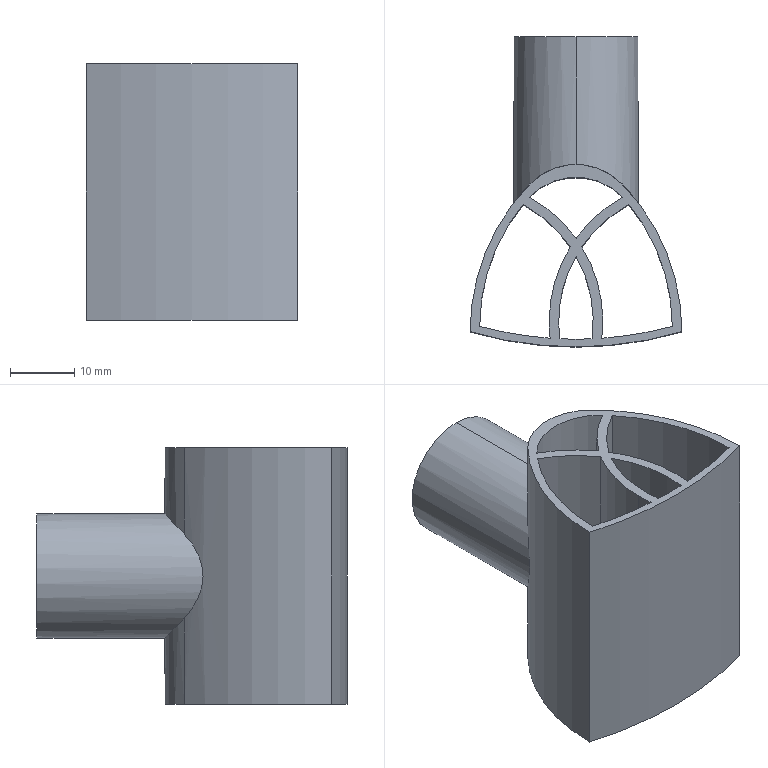Part | SolidWorks | features ICE 2, Extrusion 1 | 1 solid | 31 faces | box 33 x 48.321 x 40 mm | volume 10302 mm3 | cylinder 28 | plane 3 | commonest cylinder face diameters 41.207 x5 44.207 x5 20 x4 66 x4 114.5 x3 16 x2
STEP:
#1=CARTESIAN_POINT('',(-4.179,2.768,20.));
#2=VERTEX_POINT('',#1);
#3=CARTESIAN_POINT('',(-4.023,0.1415,20.));
#4=VERTEX_POINT('',#3);
#5=CARTESIAN_POINT('',(17.924,2.768,20.));
#6=DIRECTION('',(0.,0.,1.));
#7=DIRECTION('',(1.,0.,0.));
#8=AXIS2_PLACEMENT_3D('',#5,#6,#7);
#9=CIRCLE('',#8,22.103);
#10=EDGE_CURVE('',#2,#4,#9,.T.);
#11=ORIENTED_EDGE('',*,*,#10,.F.);
#12=CARTESIAN_POINT('',(-4.179,2.768,-20.));
#13=VERTEX_POINT('',#12);
#14=CARTESIAN_POINT('',(-4.179,2.768,20.));
#15=DIRECTION('',(0.,0.,-1.));
#16=VECTOR('',#15,1000.);
#17=LINE('',#14,#16);
#18=EDGE_CURVE('',#2,#13,#17,.T.);
#19=ORIENTED_EDGE('',*,*,#18,.T.);
#20=CARTESIAN_POINT('',(-4.023,0.1415,-20.));
#21=VERTEX_POINT('',#20);
#22=CARTESIAN_POINT('',(17.924,2.768,-20.));
#23=DIRECTION('',(0.,0.,1.));
#24=DIRECTION('',(1.,0.,0.));
#25=AXIS2_PLACEMENT_3D('',#22,#23,#24);
#26=CIRCLE('',#25,22.103);
#27=EDGE_CURVE('',#13,#21,#26,.T.);
#28=ORIENTED_EDGE('',*,*,#27,.T.);
#29=CARTESIAN_POINT('',(-4.023,0.1415,20.));
#30=DIRECTION('',(0.,0.,-1.));
#31=VECTOR('',#30,1000.);
#32=LINE('',#29,#31);
#33=EDGE_CURVE('',#4,#21,#32,.T.);
#34=ORIENTED_EDGE('',*,*,#33,.F.);
#35=EDGE_LOOP('',(#11,#19,#28,#34));
#36=FACE_OUTER_BOUND('',#35,.T.);
#37=CARTESIAN_POINT('',(17.924,2.768,20.));
#38=DIRECTION('',(0.,0.,-1.));
#39=DIRECTION('',(-1.,0.,0.));
#40=AXIS2_PLACEMENT_3D('',#37,#38,#39);
#41=CYLINDRICAL_SURFACE('',#40,22.103);
#42=ADVANCED_FACE('',(#36),#41,.T.);
#43=CARTESIAN_POINT('',(0.,12.928,20.));
#44=VERTEX_POINT('',#43);
#45=CARTESIAN_POINT('',(-2.679,2.768,20.));
#46=VERTEX_POINT('',#45);
#47=CARTESIAN_POINT('',(17.924,2.768,20.));
#48=DIRECTION('',(0.,0.,1.));
#49=DIRECTION('',(1.,0.,0.));
#50=AXIS2_PLACEMENT_3D('',#47,#48,#49);
#51=CIRCLE('',#50,20.603);
#52=EDGE_CURVE('',#44,#46,#51,.T.);
#53=ORIENTED_EDGE('',*,*,#52,.T.);
#54=CARTESIAN_POINT('',(-2.679,2.768,-20.));
#55=VERTEX_POINT('',#54);
#56=CARTESIAN_POINT('',(-2.679,2.768,20.));
#57=DIRECTION('',(0.,0.,-1.));
#58=VECTOR('',#57,1000.);
#59=LINE('',#56,#58);
#60=EDGE_CURVE('',#46,#55,#59,.T.);
#61=ORIENTED_EDGE('',*,*,#60,.T.);
#62=CARTESIAN_POINT('',(0.,12.928,-20.));
#63=VERTEX_POINT('',#62);
#64=CARTESIAN_POINT('',(17.924,2.768,-20.));
#65=DIRECTION('',(0.,0.,1.));
#66=DIRECTION('',(1.,0.,0.));
#67=AXIS2_PLACEMENT_3D('',#64,#65,#66);
#68=CIRCLE('',#67,20.603);
#69=EDGE_CURVE('',#63,#55,#68,.T.);
#70=ORIENTED_EDGE('',*,*,#69,.F.);
#71=CARTESIAN_POINT('',(0.,12.928,20.));
#72=DIRECTION('',(0.,0.,-1.));
#73=VECTOR('',#72,1000.);
#74=LINE('',#71,#73);
#75=EDGE_CURVE('',#44,#63,#74,.T.);
#76=ORIENTED_EDGE('',*,*,#75,.F.);
#77=EDGE_LOOP('',(#53,#61,#70,#76));
#78=FACE_OUTER_BOUND('',#77,.T.);
#79=CARTESIAN_POINT('',(17.924,2.768,20.));
#80=DIRECTION('',(0.,0.,-1.));
#81=DIRECTION('',(-1.,0.,0.));
#82=AXIS2_PLACEMENT_3D('',#79,#80,#81);
#83=CYLINDRICAL_SURFACE('',#82,20.603);
#84=ADVANCED_FACE('',(#78),#83,.F.);
#85=CARTESIAN_POINT('',(0.,27.201,-8.));
#86=VERTEX_POINT('',#85);
#87=CARTESIAN_POINT('',(-7.174,24.167,-3.54));
#88=VERTEX_POINT('',#87);
#89=CARTESIAN_POINT('',(0.,27.201,-8.));
#90=CARTESIAN_POINT('',(-0.3938,27.201,-8.));
#91=CARTESIAN_POINT('',(-0.7853,27.177,-7.971));
#92=CARTESIAN_POINT('',(-1.369,27.108,-7.884));
#93=CARTESIAN_POINT('',(-1.564,27.08,-7.848));
#94=CARTESIAN_POINT('',(-1.945,27.012,-7.762));
#95=CARTESIAN_POINT('',(-2.133,26.972,-7.713));
#96=CARTESIAN_POINT('',(-2.685,26.841,-7.546));
#97=CARTESIAN_POINT('',(-3.04,26.734,-7.41));
#98=CARTESIAN_POINT('',(-3.726,26.488,-7.089));
#99=CARTESIAN_POINT('',(-4.051,26.35,-6.908));
#100=CARTESIAN_POINT('',(-4.971,25.905,-6.311));
#101=CARTESIAN_POINT('',(-5.519,25.561,-5.835));
#102=CARTESIAN_POINT('',(-6.221,25.035,-5.042));
#103=CARTESIAN_POINT('',(-6.437,24.858,-4.764));
#104=CARTESIAN_POINT('',(-6.833,24.507,-4.176));
#105=CARTESIAN_POINT('',(-7.014,24.332,-3.865));
#106=CARTESIAN_POINT('',(-7.174,24.167,-3.54));
#107=B_SPLINE_CURVE_WITH_KNOTS('',3,(#89,#90,#91,#92,#93,#94,#95,#96,#97,#98,#99,#100,#101,#102,#103,#104,#105,#106),.UNSPECIFIED.,.F.,.F.,(4,2,2,2,2,2,2,2,4),(0.009445,0.01062,0.01121,0.0118,0.01297,0.01415,0.0165,0.01767,0.01885),.UNSPECIFIED.);
#108=EDGE_CURVE('',#86,#88,#107,.T.);
#109=ORIENTED_EDGE('',*,*,#108,.F.);
#110=CARTESIAN_POINT('',(0.,47.121,-8.));
#111=VERTEX_POINT('',#110);
#112=CARTESIAN_POINT('',(0.,-1.201,-8.));
#113=DIRECTION('',(0.,1.,0.));
#114=VECTOR('',#113,1000.);
#115=LINE('',#112,#114);
#116=EDGE_CURVE('',#86,#111,#115,.T.);
#117=ORIENTED_EDGE('',*,*,#116,.T.);
#118=CARTESIAN_POINT('',(0.,47.121,8.));
#119=VERTEX_POINT('',#118);
#120=CARTESIAN_POINT('',(0.,47.121,0.));
#121=DIRECTION('',(0.,-1.,0.));
#122=DIRECTION('',(0.,0.,-1.));
#123=AXIS2_PLACEMENT_3D('',#120,#121,#122);
#124=CIRCLE('',#123,8.);
#125=EDGE_CURVE('',#119,#111,#124,.T.);
#126=ORIENTED_EDGE('',*,*,#125,.F.);
#127=CARTESIAN_POINT('',(0.,27.201,8.));
#128=VERTEX_POINT('',#127);
#129=CARTESIAN_POINT('',(0.,-1.201,8.));
#130=DIRECTION('',(0.,1.,0.));
#131=VECTOR('',#130,1000.);
#132=LINE('',#129,#131);
#133=EDGE_CURVE('',#128,#119,#132,.T.);
#134=ORIENTED_EDGE('',*,*,#133,.F.);
#135=CARTESIAN_POINT('',(-7.174,24.167,3.54));
#136=VERTEX_POINT('',#135);
#137=CARTESIAN_POINT('',(-7.174,24.167,3.54));
#138=CARTESIAN_POINT('',(-6.852,24.498,4.192));
#139=CARTESIAN_POINT('',(-6.459,24.857,4.773));
#140=CARTESIAN_POINT('',(-5.756,25.383,5.567));
#141=CARTESIAN_POINT('',(-5.501,25.558,5.82));
#142=CARTESIAN_POINT('',(-4.956,25.892,6.29));
#143=CARTESIAN_POINT('',(-4.668,26.051,6.507));
#144=CARTESIAN_POINT('',(-4.059,26.346,6.903));
#145=CARTESIAN_POINT('',(-3.738,26.483,7.083));
#146=CARTESIAN_POINT('',(-3.059,26.728,7.402));
#147=CARTESIAN_POINT('',(-2.697,26.838,7.542));
#148=CARTESIAN_POINT('',(-1.957,27.015,7.767));
#149=CARTESIAN_POINT('',(-1.577,27.083,7.853));
#150=CARTESIAN_POINT('',(-0.7976,27.177,7.97));
#151=CARTESIAN_POINT('',(-0.3955,27.201,8.));
#152=CARTESIAN_POINT('',(0.,27.201,8.));
#153=B_SPLINE_CURVE_WITH_KNOTS('',3,(#137,#138,#139,#140,#141,#142,#143,#144,#145,#146,#147,#148,#149,#150,#151,#152),.UNSPECIFIED.,.F.,.F.,(4,2,2,2,2,2,2,4),(0.,0.002361,0.003542,0.004722,0.005903,0.007083,0.008264,0.009445),.UNSPECIFIED.);
#154=EDGE_CURVE('',#136,#128,#153,.T.);
#155=ORIENTED_EDGE('',*,*,#154,.F.);
#156=CARTESIAN_POINT('',(-7.174,24.167,3.54));
#157=CARTESIAN_POINT('',(-7.431,23.903,3.02));
#158=CARTESIAN_POINT('',(-7.636,23.683,2.465));
#159=CARTESIAN_POINT('',(-7.852,23.449,1.565));
#160=CARTESIAN_POINT('',(-7.907,23.388,1.256));
#161=CARTESIAN_POINT('',(-7.981,23.306,0.6372));
#162=CARTESIAN_POINT('',(-8.,23.285,0.324));
#163=CARTESIAN_POINT('',(-8.,23.285,-0.3096));
#164=CARTESIAN_POINT('',(-7.981,23.306,-0.6302));
#165=CARTESIAN_POINT('',(-7.908,23.387,-1.252));
#166=CARTESIAN_POINT('',(-7.853,23.447,-1.557));
#167=CARTESIAN_POINT('',(-7.71,23.602,-2.156));
#168=CARTESIAN_POINT('',(-7.622,23.698,-2.449));
#169=CARTESIAN_POINT('',(-7.418,23.914,-3.01));
#170=CARTESIAN_POINT('',(-7.302,24.035,-3.28));
#171=CARTESIAN_POINT('',(-7.174,24.167,-3.54));
#172=B_SPLINE_CURVE_WITH_KNOTS('',3,(#156,#157,#158,#159,#160,#161,#162,#163,#164,#165,#166,#167,#168,#169,#170,#171),.UNSPECIFIED.,.F.,.F.,(4,2,2,2,2,2,2,4),(0.,0.001893,0.00284,0.003787,0.004734,0.00568,0.006627,0.007574),.UNSPECIFIED.);
#173=EDGE_CURVE('',#136,#88,#172,.T.);
#174=ORIENTED_EDGE('',*,*,#173,.T.);
#175=EDGE_LOOP('',(#109,#117,#126,#134,#155,#174));
#176=FACE_OUTER_BOUND('',#175,.T.);
#177=CARTESIAN_POINT('',(0.,-1.201,0.));
#178=DIRECTION('',(0.,1.,0.));
#179=DIRECTION('',(0.,0.,1.));
#180=AXIS2_PLACEMENT_3D('',#177,#178,#179);
#181=CYLINDRICAL_SURFACE('',#180,8.);
#182=ADVANCED_FACE('',(#176),#181,.F.);
#183=CARTESIAN_POINT('',(7.174,24.167,-6.529));
#184=VERTEX_POINT('',#183);
#185=CARTESIAN_POINT('',(0.,27.201,-9.7));
#186=VERTEX_POINT('',#185);
#187=CARTESIAN_POINT('',(7.174,24.167,-6.529));
#188=CARTESIAN_POINT('',(6.767,24.586,-6.976));
#189=CARTESIAN_POINT('',(6.315,24.98,-7.39));
#190=CARTESIAN_POINT('',(5.556,25.521,-7.958));
#191=CARTESIAN_POINT('',(5.289,25.694,-8.138));
#192=CARTESIAN_POINT('',(4.725,26.02,-8.478));
#193=CARTESIAN_POINT('',(4.429,26.173,-8.636));
#194=CARTESIAN_POINT('',(3.818,26.449,-8.923));
#195=CARTESIAN_POINT('',(3.501,26.574,-9.053));
#196=CARTESIAN_POINT('',(2.844,26.794,-9.28));
#197=CARTESIAN_POINT('',(2.5,26.89,-9.379));
#198=CARTESIAN_POINT('',(1.45,27.121,-9.618));
#199=CARTESIAN_POINT('',(0.7337,27.201,-9.7));
#200=CARTESIAN_POINT('',(0.,27.201,-9.7));
#201=B_SPLINE_CURVE_WITH_KNOTS('',3,(#187,#188,#189,#190,#191,#192,#193,#194,#195,#196,#197,#198,#199,#200),.UNSPECIFIED.,.F.,.F.,(4,2,2,2,2,2,4),(0.,0.002182,0.003273,0.004364,0.005455,0.006546,0.008728),.UNSPECIFIED.);
#202=EDGE_CURVE('',#184,#186,#201,.T.);
#203=ORIENTED_EDGE('',*,*,#202,.T.);
#204=CARTESIAN_POINT('',(0.,47.121,-9.7));
#205=VERTEX_POINT('',#204);
#206=CARTESIAN_POINT('',(0.,-1.201,-9.7));
#207=DIRECTION('',(0.,1.,0.));
#208=VECTOR('',#207,1000.);
#209=LINE('',#206,#208);
#210=EDGE_CURVE('',#186,#205,#209,.T.);
#211=ORIENTED_EDGE('',*,*,#210,.T.);
#212=CARTESIAN_POINT('',(0.,47.121,9.7));
#213=VERTEX_POINT('',#212);
#214=CARTESIAN_POINT('',(0.,47.121,0.));
#215=DIRECTION('',(0.,-1.,0.));
#216=DIRECTION('',(0.,0.,-1.));
#217=AXIS2_PLACEMENT_3D('',#214,#215,#216);
#218=CIRCLE('',#217,9.7);
#219=EDGE_CURVE('',#205,#213,#218,.T.);
#220=ORIENTED_EDGE('',*,*,#219,.T.);
#221=CARTESIAN_POINT('',(0.,27.201,9.7));
#222=VERTEX_POINT('',#221);
#223=CARTESIAN_POINT('',(0.,-1.201,9.7));
#224=DIRECTION('',(0.,1.,0.));
#225=VECTOR('',#224,1000.);
#226=LINE('',#223,#225);
#227=EDGE_CURVE('',#222,#213,#226,.T.);
#228=ORIENTED_EDGE('',*,*,#227,.F.);
#229=CARTESIAN_POINT('',(7.174,24.167,6.529));
#230=VERTEX_POINT('',#229);
#231=CARTESIAN_POINT('',(0.,27.201,9.7));
#232=CARTESIAN_POINT('',(0.366,27.201,9.7));
#233=CARTESIAN_POINT('',(0.7354,27.18,9.679));
#234=CARTESIAN_POINT('',(1.455,27.101,9.597));
#235=CARTESIAN_POINT('',(1.809,27.042,9.537));
#236=CARTESIAN_POINT('',(2.505,26.888,9.378));
#237=CARTESIAN_POINT('',(2.849,26.792,9.279));
#238=CARTESIAN_POINT('',(3.508,26.572,9.05));
#239=CARTESIAN_POINT('',(3.825,26.446,8.92));
#240=CARTESIAN_POINT('',(4.436,26.169,8.633));
#241=CARTESIAN_POINT('',(4.732,26.016,8.474));
#242=CARTESIAN_POINT('',(5.294,25.691,8.135));
#243=CARTESIAN_POINT('',(5.559,25.519,7.955));
#244=CARTESIAN_POINT('',(6.316,24.978,7.389));
#245=CARTESIAN_POINT('',(6.768,24.586,6.975));
#246=CARTESIAN_POINT('',(7.174,24.167,6.529));
#247=B_SPLINE_CURVE_WITH_KNOTS('',3,(#231,#232,#233,#234,#235,#236,#237,#238,#239,#240,#241,#242,#243,#244,#245,#246),.UNSPECIFIED.,.F.,.F.,(4,2,2,2,2,2,2,4),(0.008728,0.009816,0.0109,0.01199,0.01308,0.01417,0.01526,0.01743),.UNSPECIFIED.);
#248=EDGE_CURVE('',#222,#230,#247,.T.);
#249=ORIENTED_EDGE('',*,*,#248,.T.);
#250=CARTESIAN_POINT('',(7.174,24.167,6.529));
#251=CARTESIAN_POINT('',(7.538,23.793,6.129));
#252=CARTESIAN_POINT('',(7.87,23.433,5.697));
#253=CARTESIAN_POINT('',(8.32,22.926,4.994));
#254=CARTESIAN_POINT('',(8.462,22.763,4.75));
#255=CARTESIAN_POINT('',(8.729,22.45,4.24));
#256=CARTESIAN_POINT('',(8.854,22.301,3.973));
#257=CARTESIAN_POINT('',(9.195,21.888,3.147));
#258=CARTESIAN_POINT('',(9.377,21.657,2.564));
#259=CARTESIAN_POINT('',(9.568,21.412,1.624));
#260=CARTESIAN_POINT('',(9.617,21.349,1.304));
#261=CARTESIAN_POINT('',(9.683,21.264,0.6603));
#262=CARTESIAN_POINT('',(9.7,21.241,0.3346));
#263=CARTESIAN_POINT('',(9.7,21.241,-0.3247));
#264=CARTESIAN_POINT('',(9.683,21.263,-0.6547));
#265=CARTESIAN_POINT('',(9.618,21.348,-1.299));
#266=CARTESIAN_POINT('',(9.57,21.41,-1.617));
#267=CARTESIAN_POINT('',(9.443,21.573,-2.241));
#268=CARTESIAN_POINT('',(9.364,21.672,-2.548));
#269=CARTESIAN_POINT('',(9.185,21.897,-3.134));
#270=CARTESIAN_POINT('',(9.083,22.023,-3.417));
#271=CARTESIAN_POINT('',(8.745,22.433,-4.239));
#272=CARTESIAN_POINT('',(8.474,22.753,-4.753));
#273=CARTESIAN_POINT('',(7.871,23.431,-5.696));
#274=CARTESIAN_POINT('',(7.538,23.792,-6.129));
#275=CARTESIAN_POINT('',(7.174,24.167,-6.529));
#276=B_SPLINE_CURVE_WITH_KNOTS('',3,(#250,#251,#252,#253,#254,#255,#256,#257,#258,#259,#260,#261,#262,#263,#264,#265,#266,#267,#268,#269,#270,#271,#272,#273,#274,#275),.UNSPECIFIED.,.F.,.F.,(4,2,2,2,2,2,2,2,2,2,2,2,4),(0.,0.001953,0.00293,0.003907,0.00586,0.006837,0.007814,0.008791,0.009767,0.01074,0.01172,0.01367,0.01563),.UNSPECIFIED.);
#277=EDGE_CURVE('',#230,#184,#276,.T.);
#278=ORIENTED_EDGE('',*,*,#277,.T.);
#279=EDGE_LOOP('',(#203,#211,#220,#228,#249,#278));
#280=FACE_OUTER_BOUND('',#279,.T.);
#281=CARTESIAN_POINT('',(0.,-1.201,0.));
#282=DIRECTION('',(0.,1.,0.));
#283=DIRECTION('',(0.,0.,1.));
#284=AXIS2_PLACEMENT_3D('',#281,#282,#283);
#285=CYLINDRICAL_SURFACE('',#284,9.7);
#286=ADVANCED_FACE('',(#280),#285,.T.);
#287=ORIENTED_EDGE('',*,*,#277,.F.);
#288=CARTESIAN_POINT('',(7.174,24.167,20.));
#289=VERTEX_POINT('',#288);
#290=CARTESIAN_POINT('',(7.174,24.167,20.));
#291=DIRECTION('',(0.,0.,-1.));
#292=VECTOR('',#291,1000.);
#293=LINE('',#290,#292);
#294=EDGE_CURVE('',#289,#230,#293,.T.);
#295=ORIENTED_EDGE('',*,*,#294,.F.);
#296=CARTESIAN_POINT('',(16.5,1.177,20.));
#297=VERTEX_POINT('',#296);
#298=CARTESIAN_POINT('',(-16.5,1.177,20.));
#299=DIRECTION('',(0.,0.,1.));
#300=DIRECTION('',(1.,0.,0.));
#301=AXIS2_PLACEMENT_3D('',#298,#299,#300);
#302=CIRCLE('',#301,33.);
#303=EDGE_CURVE('',#297,#289,#302,.T.);
#304=ORIENTED_EDGE('',*,*,#303,.F.);
#305=CARTESIAN_POINT('',(16.5,1.177,-20.));
#306=VERTEX_POINT('',#305);
#307=CARTESIAN_POINT('',(16.5,1.177,20.));
#308=DIRECTION('',(0.,0.,-1.));
#309=VECTOR('',#308,1000.);
#310=LINE('',#307,#309);
#311=EDGE_CURVE('',#297,#306,#310,.T.);
#312=ORIENTED_EDGE('',*,*,#311,.T.);
#313=CARTESIAN_POINT('',(7.174,24.167,-20.));
#314=VERTEX_POINT('',#313);
#315=CARTESIAN_POINT('',(-16.5,1.177,-20.));
#316=DIRECTION('',(0.,0.,1.));
#317=DIRECTION('',(1.,0.,0.));
#318=AXIS2_PLACEMENT_3D('',#315,#316,#317);
#319=CIRCLE('',#318,33.);
#320=EDGE_CURVE('',#306,#314,#319,.T.);
#321=ORIENTED_EDGE('',*,*,#320,.T.);
#322=CARTESIAN_POINT('',(7.174,24.167,20.));
#323=DIRECTION('',(0.,0.,-1.));
#324=VECTOR('',#323,1000.);
#325=LINE('',#322,#324);
#326=EDGE_CURVE('',#184,#314,#325,.T.);
#327=ORIENTED_EDGE('',*,*,#326,.F.);
#328=EDGE_LOOP('',(#287,#295,#304,#312,#321,#327));
#329=FACE_OUTER_BOUND('',#328,.T.);
#330=CARTESIAN_POINT('',(-16.5,1.177,20.));
#331=DIRECTION('',(0.,0.,-1.));
#332=DIRECTION('',(-1.,0.,0.));
#333=AXIS2_PLACEMENT_3D('',#330,#331,#332);
#334=CYLINDRICAL_SURFACE('',#333,33.);
#335=ADVANCED_FACE('',(#329),#334,.T.);
#336=ORIENTED_EDGE('',*,*,#202,.F.);
#337=ORIENTED_EDGE('',*,*,#326,.T.);
#338=CARTESIAN_POINT('',(-7.174,24.167,-20.));
#339=VERTEX_POINT('',#338);
#340=CARTESIAN_POINT('',(0.,17.201,-20.));
#341=DIRECTION('',(0.,0.,1.));
#342=DIRECTION('',(1.,0.,0.));
#343=AXIS2_PLACEMENT_3D('',#340,#341,#342);
#344=CIRCLE('',#343,10.);
#345=EDGE_CURVE('',#314,#339,#344,.T.);
#346=ORIENTED_EDGE('',*,*,#345,.T.);
#347=CARTESIAN_POINT('',(-7.174,24.167,-6.529));
#348=VERTEX_POINT('',#347);
#349=CARTESIAN_POINT('',(-7.174,24.167,20.));
#350=DIRECTION('',(0.,0.,-1.));
#351=VECTOR('',#350,1000.);
#352=LINE('',#349,#351);
#353=EDGE_CURVE('',#348,#339,#352,.T.);
#354=ORIENTED_EDGE('',*,*,#353,.F.);
#355=CARTESIAN_POINT('',(0.,27.201,-9.7));
#356=CARTESIAN_POINT('',(-0.366,27.201,-9.7));
#357=CARTESIAN_POINT('',(-0.7354,27.18,-9.679));
#358=CARTESIAN_POINT('',(-1.455,27.101,-9.597));
#359=CARTESIAN_POINT('',(-1.809,27.042,-9.537));
#360=CARTESIAN_POINT('',(-2.505,26.888,-9.378));
#361=CARTESIAN_POINT('',(-2.849,26.792,-9.279));
#362=CARTESIAN_POINT('',(-3.508,26.572,-9.05));
#363=CARTESIAN_POINT('',(-3.825,26.446,-8.92));
#364=CARTESIAN_POINT('',(-4.436,26.169,-8.633));
#365=CARTESIAN_POINT('',(-4.732,26.016,-8.474));
#366=CARTESIAN_POINT('',(-5.294,25.691,-8.135));
#367=CARTESIAN_POINT('',(-5.559,25.519,-7.955));
#368=CARTESIAN_POINT('',(-6.316,24.978,-7.389));
#369=CARTESIAN_POINT('',(-6.768,24.586,-6.975));
#370=CARTESIAN_POINT('',(-7.174,24.167,-6.529));
#371=B_SPLINE_CURVE_WITH_KNOTS('',3,(#355,#356,#357,#358,#359,#360,#361,#362,#363,#364,#365,#366,#367,#368,#369,#370),.UNSPECIFIED.,.F.,.F.,(4,2,2,2,2,2,2,4),(0.008728,0.009816,0.0109,0.01199,0.01308,0.01417,0.01526,0.01743),.UNSPECIFIED.);
#372=EDGE_CURVE('',#186,#348,#371,.T.);
#373=ORIENTED_EDGE('',*,*,#372,.F.);
#374=EDGE_LOOP('',(#336,#337,#346,#354,#373));
#375=FACE_OUTER_BOUND('',#374,.T.);
#376=CARTESIAN_POINT('',(0.,17.201,20.));
#377=DIRECTION('',(0.,0.,-1.));
#378=DIRECTION('',(-1.,0.,0.));
#379=AXIS2_PLACEMENT_3D('',#376,#377,#378);
#380=CYLINDRICAL_SURFACE('',#379,10.);
#381=ADVANCED_FACE('',(#375),#380,.T.);
#382=CARTESIAN_POINT('',(-7.174,24.167,6.529));
#383=VERTEX_POINT('',#382);
#384=CARTESIAN_POINT('',(-7.174,24.167,6.529));
#385=CARTESIAN_POINT('',(-6.767,24.586,6.976));
#386=CARTESIAN_POINT('',(-6.315,24.98,7.39));
#387=CARTESIAN_POINT('',(-5.556,25.521,7.958));
#388=CARTESIAN_POINT('',(-5.289,25.694,8.138));
#389=CARTESIAN_POINT('',(-4.725,26.02,8.478));
#390=CARTESIAN_POINT('',(-4.429,26.173,8.636));
#391=CARTESIAN_POINT('',(-3.818,26.449,8.923));
#392=CARTESIAN_POINT('',(-3.501,26.574,9.053));
#393=CARTESIAN_POINT('',(-2.844,26.794,9.28));
#394=CARTESIAN_POINT('',(-2.5,26.89,9.379));
#395=CARTESIAN_POINT('',(-1.45,27.121,9.618));
#396=CARTESIAN_POINT('',(-0.7337,27.201,9.7));
#397=CARTESIAN_POINT('',(0.,27.201,9.7));
#398=B_SPLINE_CURVE_WITH_KNOTS('',3,(#384,#385,#386,#387,#388,#389,#390,#391,#392,#393,#394,#395,#396,#397),.UNSPECIFIED.,.F.,.F.,(4,2,2,2,2,2,4),(0.,0.002182,0.003273,0.004364,0.005455,0.006546,0.008728),.UNSPECIFIED.);
#399=EDGE_CURVE('',#383,#222,#398,.T.);
#400=ORIENTED_EDGE('',*,*,#399,.F.);
#401=CARTESIAN_POINT('',(-7.174,24.167,20.));
#402=VERTEX_POINT('',#401);
#403=CARTESIAN_POINT('',(-7.174,24.167,20.));
#404=DIRECTION('',(0.,0.,-1.));
#405=VECTOR('',#404,1000.);
#406=LINE('',#403,#405);
#407=EDGE_CURVE('',#402,#383,#406,.T.);
#408=ORIENTED_EDGE('',*,*,#407,.F.);
#409=CARTESIAN_POINT('',(0.,17.201,20.));
#410=DIRECTION('',(0.,0.,1.));
#411=DIRECTION('',(1.,0.,0.));
#412=AXIS2_PLACEMENT_3D('',#409,#410,#411);
#413=CIRCLE('',#412,10.);
#414=EDGE_CURVE('',#289,#402,#413,.T.);
#415=ORIENTED_EDGE('',*,*,#414,.F.);
#416=ORIENTED_EDGE('',*,*,#294,.T.);
#417=ORIENTED_EDGE('',*,*,#248,.F.);
#418=EDGE_LOOP('',(#400,#408,#415,#416,#417));
#419=FACE_OUTER_BOUND('',#418,.T.);
#420=CARTESIAN_POINT('',(0.,17.201,20.));
#421=DIRECTION('',(0.,0.,-1.));
#422=DIRECTION('',(-1.,0.,0.));
#423=AXIS2_PLACEMENT_3D('',#420,#421,#422);
#424=CYLINDRICAL_SURFACE('',#423,10.);
#425=ADVANCED_FACE('',(#419),#424,.T.);
#426=ORIENTED_EDGE('',*,*,#407,.T.);
#427=CARTESIAN_POINT('',(-7.174,24.167,6.529));
#428=CARTESIAN_POINT('',(-7.538,23.793,6.129));
#429=CARTESIAN_POINT('',(-7.87,23.433,5.697));
#430=CARTESIAN_POINT('',(-8.32,22.926,4.994));
#431=CARTESIAN_POINT('',(-8.462,22.763,4.75));
#432=CARTESIAN_POINT('',(-8.729,22.45,4.24));
#433=CARTESIAN_POINT('',(-8.854,22.301,3.973));
#434=CARTESIAN_POINT('',(-9.195,21.888,3.147));
#435=CARTESIAN_POINT('',(-9.377,21.657,2.564));
#436=CARTESIAN_POINT('',(-9.568,21.412,1.624));
#437=CARTESIAN_POINT('',(-9.617,21.349,1.304));
#438=CARTESIAN_POINT('',(-9.683,21.264,0.6603));
#439=CARTESIAN_POINT('',(-9.7,21.241,0.3346));
#440=CARTESIAN_POINT('',(-9.7,21.241,-0.3247));
#441=CARTESIAN_POINT('',(-9.683,21.263,-0.6547));
#442=CARTESIAN_POINT('',(-9.618,21.348,-1.299));
#443=CARTESIAN_POINT('',(-9.57,21.41,-1.617));
#444=CARTESIAN_POINT('',(-9.443,21.573,-2.241));
#445=CARTESIAN_POINT('',(-9.364,21.672,-2.548));
#446=CARTESIAN_POINT('',(-9.185,21.897,-3.134));
#447=CARTESIAN_POINT('',(-9.083,22.023,-3.417));
#448=CARTESIAN_POINT('',(-8.745,22.433,-4.239));
#449=CARTESIAN_POINT('',(-8.474,22.753,-4.753));
#450=CARTESIAN_POINT('',(-7.871,23.431,-5.696));
#451=CARTESIAN_POINT('',(-7.538,23.792,-6.129));
#452=CARTESIAN_POINT('',(-7.174,24.167,-6.529));
#453=B_SPLINE_CURVE_WITH_KNOTS('',3,(#427,#428,#429,#430,#431,#432,#433,#434,#435,#436,#437,#438,#439,#440,#441,#442,#443,#444,#445,#446,#447,#448,#449,#450,#451,#452),.UNSPECIFIED.,.F.,.F.,(4,2,2,2,2,2,2,2,2,2,2,2,4),(0.,0.001953,0.00293,0.003907,0.00586,0.006837,0.007814,0.008791,0.009767,0.01074,0.01172,0.01367,0.01563),.UNSPECIFIED.);
#454=EDGE_CURVE('',#383,#348,#453,.T.);
#455=ORIENTED_EDGE('',*,*,#454,.T.);
#456=ORIENTED_EDGE('',*,*,#353,.T.);
#457=CARTESIAN_POINT('',(-16.5,1.177,-20.));
#458=VERTEX_POINT('',#457);
#459=CARTESIAN_POINT('',(16.5,1.177,-20.));
#460=DIRECTION('',(0.,0.,-1.));
#461=DIRECTION('',(1.,0.,0.));
#462=AXIS2_PLACEMENT_3D('',#459,#460,#461);
#463=CIRCLE('',#462,33.);
#464=EDGE_CURVE('',#458,#339,#463,.T.);
#465=ORIENTED_EDGE('',*,*,#464,.F.);
#466=CARTESIAN_POINT('',(-16.5,1.177,20.));
#467=VERTEX_POINT('',#466);
#468=CARTESIAN_POINT('',(-16.5,1.177,20.));
#469=DIRECTION('',(0.,0.,-1.));
#470=VECTOR('',#469,1000.);
#471=LINE('',#468,#470);
#472=EDGE_CURVE('',#467,#458,#471,.T.);
#473=ORIENTED_EDGE('',*,*,#472,.F.);
#474=CARTESIAN_POINT('',(16.5,1.177,20.));
#475=DIRECTION('',(0.,0.,-1.));
#476=DIRECTION('',(1.,0.,0.));
#477=AXIS2_PLACEMENT_3D('',#474,#475,#476);
#478=CIRCLE('',#477,33.);
#479=EDGE_CURVE('',#467,#402,#478,.T.);
#480=ORIENTED_EDGE('',*,*,#479,.T.);
#481=EDGE_LOOP('',(#426,#455,#456,#465,#473,#480));
#482=FACE_OUTER_BOUND('',#481,.T.);
#483=CARTESIAN_POINT('',(16.5,1.177,20.));
#484=DIRECTION('',(0.,0.,-1.));
#485=DIRECTION('',(-1.,0.,0.));
#486=AXIS2_PLACEMENT_3D('',#483,#484,#485);
#487=CYLINDRICAL_SURFACE('',#486,33.);
#488=ADVANCED_FACE('',(#482),#487,.T.);
#489=CARTESIAN_POINT('',(-15.,2.,-20.));
#490=VERTEX_POINT('',#489);
#491=CARTESIAN_POINT('',(-8.25,20.959,-20.));
#492=VERTEX_POINT('',#491);
#493=CARTESIAN_POINT('',(15.,2.,-20.));
#494=DIRECTION('',(0.,0.,-1.));
#495=DIRECTION('',(1.,0.,0.));
#496=AXIS2_PLACEMENT_3D('',#493,#494,#495);
#497=CIRCLE('',#496,30.);
#498=EDGE_CURVE('',#490,#492,#497,.T.);
#499=ORIENTED_EDGE('',*,*,#498,.T.);
#500=CARTESIAN_POINT('',(-8.25,20.959,20.));
#501=VERTEX_POINT('',#500);
#502=CARTESIAN_POINT('',(-8.25,20.959,20.));
#503=DIRECTION('',(0.,0.,-1.));
#504=VECTOR('',#503,1000.);
#505=LINE('',#502,#504);
#506=EDGE_CURVE('',#501,#492,#505,.T.);
#507=ORIENTED_EDGE('',*,*,#506,.F.);
#508=CARTESIAN_POINT('',(-15.,2.,20.));
#509=VERTEX_POINT('',#508);
#510=CARTESIAN_POINT('',(15.,2.,20.));
#511=DIRECTION('',(0.,0.,-1.));
#512=DIRECTION('',(1.,0.,0.));
#513=AXIS2_PLACEMENT_3D('',#510,#511,#512);
#514=CIRCLE('',#513,30.);
#515=EDGE_CURVE('',#509,#501,#514,.T.);
#516=ORIENTED_EDGE('',*,*,#515,.F.);
#517=CARTESIAN_POINT('',(-15.,2.,20.));
#518=DIRECTION('',(0.,0.,-1.));
#519=VECTOR('',#518,1000.);
#520=LINE('',#517,#519);
#521=EDGE_CURVE('',#509,#490,#520,.T.);
#522=ORIENTED_EDGE('',*,*,#521,.T.);
#523=EDGE_LOOP('',(#499,#507,#516,#522));
#524=FACE_OUTER_BOUND('',#523,.T.);
#525=CARTESIAN_POINT('',(15.,2.,20.));
#526=DIRECTION('',(0.,0.,-1.));
#527=DIRECTION('',(-1.,0.,0.));
#528=AXIS2_PLACEMENT_3D('',#525,#526,#527);
#529=CYLINDRICAL_SURFACE('',#528,30.);
#530=ADVANCED_FACE('',(#524),#529,.F.);
#531=CARTESIAN_POINT('',(8.25,20.959,20.));
#532=VERTEX_POINT('',#531);
#533=CARTESIAN_POINT('',(8.25,20.959,-20.));
#534=VERTEX_POINT('',#533);
#535=CARTESIAN_POINT('',(8.25,20.959,20.));
#536=DIRECTION('',(0.,0.,-1.));
#537=VECTOR('',#536,1000.);
#538=LINE('',#535,#537);
#539=EDGE_CURVE('',#532,#534,#538,.T.);
#540=ORIENTED_EDGE('',*,*,#539,.T.);
#541=CARTESIAN_POINT('',(15.,2.,-20.));
#542=VERTEX_POINT('',#541);
#543=CARTESIAN_POINT('',(-15.,2.,-20.));
#544=DIRECTION('',(0.,0.,1.));
#545=DIRECTION('',(1.,0.,0.));
#546=AXIS2_PLACEMENT_3D('',#543,#544,#545);
#547=CIRCLE('',#546,30.);
#548=EDGE_CURVE('',#542,#534,#547,.T.);
#549=ORIENTED_EDGE('',*,*,#548,.F.);
#550=CARTESIAN_POINT('',(15.,2.,20.));
#551=VERTEX_POINT('',#550);
#552=CARTESIAN_POINT('',(15.,2.,20.));
#553=DIRECTION('',(0.,0.,-1.));
#554=VECTOR('',#553,1000.);
#555=LINE('',#552,#554);
#556=EDGE_CURVE('',#551,#542,#555,.T.);
#557=ORIENTED_EDGE('',*,*,#556,.F.);
#558=CARTESIAN_POINT('',(-15.,2.,20.));
#559=DIRECTION('',(0.,0.,1.));
#560=DIRECTION('',(1.,0.,0.));
#561=AXIS2_PLACEMENT_3D('',#558,#559,#560);
#562=CIRCLE('',#561,30.);
#563=EDGE_CURVE('',#551,#532,#562,.T.);
#564=ORIENTED_EDGE('',*,*,#563,.T.);
#565=EDGE_LOOP('',(#540,#549,#557,#564));
#566=FACE_OUTER_BOUND('',#565,.T.);
#567=CARTESIAN_POINT('',(-15.,2.,20.));
#568=DIRECTION('',(0.,0.,-1.));
#569=DIRECTION('',(-1.,0.,0.));
#570=AXIS2_PLACEMENT_3D('',#567,#568,#569);
#571=CYLINDRICAL_SURFACE('',#570,30.);
#572=ADVANCED_FACE('',(#566),#571,.F.);
#573=CARTESIAN_POINT('',(0.,57.25,-20.));
#574=DIRECTION('',(0.,0.,1.));
#575=DIRECTION('',(1.,0.,0.));
#576=AXIS2_PLACEMENT_3D('',#573,#574,#575);
#577=CIRCLE('',#576,58.45);
#578=EDGE_CURVE('',#458,#306,#577,.T.);
#579=ORIENTED_EDGE('',*,*,#578,.T.);
#580=ORIENTED_EDGE('',*,*,#311,.F.);
#581=CARTESIAN_POINT('',(0.,57.25,20.));
#582=DIRECTION('',(0.,0.,1.));
#583=DIRECTION('',(1.,0.,0.));
#584=AXIS2_PLACEMENT_3D('',#581,#582,#583);
#585=CIRCLE('',#584,58.45);
#586=EDGE_CURVE('',#467,#297,#585,.T.);
#587=ORIENTED_EDGE('',*,*,#586,.F.);
#588=ORIENTED_EDGE('',*,*,#472,.T.);
#589=EDGE_LOOP('',(#579,#580,#587,#588));
#590=FACE_OUTER_BOUND('',#589,.T.);
#591=CARTESIAN_POINT('',(0.,57.25,20.));
#592=DIRECTION('',(0.,0.,-1.));
#593=DIRECTION('',(-1.,0.,0.));
#594=AXIS2_PLACEMENT_3D('',#591,#592,#593);
#595=CYLINDRICAL_SURFACE('',#594,58.45);
#596=ADVANCED_FACE('',(#590),#595,.T.);
#597=CARTESIAN_POINT('',(7.246,22.121,20.));
#598=VERTEX_POINT('',#597);
#599=CARTESIAN_POINT('',(-7.246,22.121,20.));
#600=VERTEX_POINT('',#599);
#601=CARTESIAN_POINT('',(0.,15.229,20.));
#602=DIRECTION('',(0.,0.,1.));
#603=DIRECTION('',(1.,0.,0.));
#604=AXIS2_PLACEMENT_3D('',#601,#602,#603);
#605=CIRCLE('',#604,10.);
#606=EDGE_CURVE('',#598,#600,#605,.T.);
#607=ORIENTED_EDGE('',*,*,#606,.F.);
#608=CARTESIAN_POINT('',(0.,15.702,20.));
#609=VERTEX_POINT('',#608);
#610=CARTESIAN_POINT('',(17.924,2.768,20.));
#611=DIRECTION('',(0.,0.,1.));
#612=DIRECTION('',(1.,0.,0.));
#613=AXIS2_PLACEMENT_3D('',#610,#611,#612);
#614=CIRCLE('',#613,22.103);
#615=EDGE_CURVE('',#598,#609,#614,.T.);
#616=ORIENTED_EDGE('',*,*,#615,.T.);
#617=CARTESIAN_POINT('',(-17.924,2.768,20.));
#618=DIRECTION('',(0.,0.,-1.));
#619=DIRECTION('',(1.,0.,0.));
#620=AXIS2_PLACEMENT_3D('',#617,#618,#619);
#621=CIRCLE('',#620,22.103);
#622=EDGE_CURVE('',#600,#609,#621,.T.);
#623=ORIENTED_EDGE('',*,*,#622,.F.);
#624=EDGE_LOOP('',(#607,#616,#623));
#625=FACE_BOUND('',#624,.T.);
#626=CARTESIAN_POINT('',(-2.5,0.05461,20.));
#627=VERTEX_POINT('',#626);
#628=CARTESIAN_POINT('',(2.5,0.05461,20.));
#629=VERTEX_POINT('',#628);
#630=CARTESIAN_POINT('',(0.,57.25,20.));
#631=DIRECTION('',(0.,0.,1.));
#632=DIRECTION('',(1.,0.,0.));
#633=AXIS2_PLACEMENT_3D('',#630,#631,#632);
#634=CIRCLE('',#633,57.25);
#635=EDGE_CURVE('',#627,#629,#634,.T.);
#636=ORIENTED_EDGE('',*,*,#635,.F.);
#637=CARTESIAN_POINT('',(17.924,2.768,20.));
#638=DIRECTION('',(0.,0.,1.));
#639=DIRECTION('',(1.,0.,0.));
#640=AXIS2_PLACEMENT_3D('',#637,#638,#639);
#641=CIRCLE('',#640,20.603);
#642=EDGE_CURVE('',#46,#627,#641,.T.);
#643=ORIENTED_EDGE('',*,*,#642,.F.);
#644=ORIENTED_EDGE('',*,*,#52,.F.);
#645=CARTESIAN_POINT('',(-17.924,2.768,20.));
#646=DIRECTION('',(0.,0.,-1.));
#647=DIRECTION('',(1.,0.,0.));
#648=AXIS2_PLACEMENT_3D('',#645,#646,#647);
#649=CIRCLE('',#648,20.603);
#650=EDGE_CURVE('',#44,#629,#649,.T.);
#651=ORIENTED_EDGE('',*,*,#650,.T.);
#652=EDGE_LOOP('',(#636,#643,#644,#651));
#653=FACE_BOUND('',#652,.T.);
#654=CARTESIAN_POINT('',(4.023,0.1415,20.));
#655=VERTEX_POINT('',#654);
#656=CARTESIAN_POINT('',(0.,57.25,20.));
#657=DIRECTION('',(0.,0.,1.));
#658=DIRECTION('',(1.,0.,0.));
#659=AXIS2_PLACEMENT_3D('',#656,#657,#658);
#660=CIRCLE('',#659,57.25);
#661=EDGE_CURVE('',#655,#551,#660,.T.);
#662=ORIENTED_EDGE('',*,*,#661,.F.);
#663=CARTESIAN_POINT('',(0.8935,14.364,20.));
#664=VERTEX_POINT('',#663);
#665=CARTESIAN_POINT('',(-17.924,2.768,20.));
#666=DIRECTION('',(0.,0.,-1.));
#667=DIRECTION('',(1.,0.,0.));
#668=AXIS2_PLACEMENT_3D('',#665,#666,#667);
#669=CIRCLE('',#668,22.103);
#670=EDGE_CURVE('',#664,#655,#669,.T.);
#671=ORIENTED_EDGE('',*,*,#670,.F.);
#672=CARTESIAN_POINT('',(17.924,2.768,20.));
#673=DIRECTION('',(0.,0.,1.));
#674=DIRECTION('',(1.,0.,0.));
#675=AXIS2_PLACEMENT_3D('',#672,#673,#674);
#676=CIRCLE('',#675,20.603);
#677=EDGE_CURVE('',#532,#664,#676,.T.);
#678=ORIENTED_EDGE('',*,*,#677,.F.);
#679=ORIENTED_EDGE('',*,*,#563,.F.);
#680=EDGE_LOOP('',(#662,#671,#678,#679));
#681=FACE_BOUND('',#680,.T.);
#682=CARTESIAN_POINT('',(-0.8935,14.364,20.));
#683=VERTEX_POINT('',#682);
#684=CARTESIAN_POINT('',(17.924,2.768,20.));
#685=DIRECTION('',(0.,0.,1.));
#686=DIRECTION('',(1.,0.,0.));
#687=AXIS2_PLACEMENT_3D('',#684,#685,#686);
#688=CIRCLE('',#687,22.103);
#689=EDGE_CURVE('',#683,#2,#688,.T.);
#690=ORIENTED_EDGE('',*,*,#689,.T.);
#691=ORIENTED_EDGE('',*,*,#10,.T.);
#692=CARTESIAN_POINT('',(0.,57.25,20.));
#693=DIRECTION('',(0.,0.,1.));
#694=DIRECTION('',(1.,0.,0.));
#695=AXIS2_PLACEMENT_3D('',#692,#693,#694);
#696=CIRCLE('',#695,57.25);
#697=EDGE_CURVE('',#509,#4,#696,.T.);
#698=ORIENTED_EDGE('',*,*,#697,.F.);
#699=ORIENTED_EDGE('',*,*,#515,.T.);
#700=CARTESIAN_POINT('',(-17.924,2.768,20.));
#701=DIRECTION('',(0.,0.,-1.));
#702=DIRECTION('',(1.,0.,0.));
#703=AXIS2_PLACEMENT_3D('',#700,#701,#702);
#704=CIRCLE('',#703,20.603);
#705=EDGE_CURVE('',#501,#683,#704,.T.);
#706=ORIENTED_EDGE('',*,*,#705,.T.);
#707=EDGE_LOOP('',(#690,#691,#698,#699,#706));
#708=FACE_BOUND('',#707,.T.);
#709=ORIENTED_EDGE('',*,*,#303,.T.);
#710=ORIENTED_EDGE('',*,*,#414,.T.);
#711=ORIENTED_EDGE('',*,*,#479,.F.);
#712=ORIENTED_EDGE('',*,*,#586,.T.);
#713=EDGE_LOOP('',(#709,#710,#711,#712));
#714=FACE_OUTER_BOUND('',#713,.T.);
#715=CARTESIAN_POINT('',(0.,0.,20.));
#716=DIRECTION('',(0.,0.,1.));
#717=DIRECTION('',(1.,0.,0.));
#718=AXIS2_PLACEMENT_3D('',#715,#716,#717);
#719=PLANE('',#718);
#720=ADVANCED_FACE('',(#625,#653,#681,#708,#714),#719,.T.);
#721=CARTESIAN_POINT('',(7.246,22.121,-20.));
#722=VERTEX_POINT('',#721);
#723=CARTESIAN_POINT('',(-7.246,22.121,-20.));
#724=VERTEX_POINT('',#723);
#725=CARTESIAN_POINT('',(0.,15.229,-20.));
#726=DIRECTION('',(0.,0.,1.));
#727=DIRECTION('',(1.,0.,0.));
#728=AXIS2_PLACEMENT_3D('',#725,#726,#727);
#729=CIRCLE('',#728,10.);
#730=EDGE_CURVE('',#722,#724,#729,.T.);
#731=ORIENTED_EDGE('',*,*,#730,.T.);
#732=CARTESIAN_POINT('',(0.,15.702,-20.));
#733=VERTEX_POINT('',#732);
#734=CARTESIAN_POINT('',(-17.924,2.768,-20.));
#735=DIRECTION('',(0.,0.,-1.));
#736=DIRECTION('',(1.,0.,0.));
#737=AXIS2_PLACEMENT_3D('',#734,#735,#736);
#738=CIRCLE('',#737,22.103);
#739=EDGE_CURVE('',#724,#733,#738,.T.);
#740=ORIENTED_EDGE('',*,*,#739,.T.);
#741=CARTESIAN_POINT('',(17.924,2.768,-20.));
#742=DIRECTION('',(0.,0.,1.));
#743=DIRECTION('',(1.,0.,0.));
#744=AXIS2_PLACEMENT_3D('',#741,#742,#743);
#745=CIRCLE('',#744,22.103);
#746=EDGE_CURVE('',#722,#733,#745,.T.);
#747=ORIENTED_EDGE('',*,*,#746,.F.);
#748=EDGE_LOOP('',(#731,#740,#747));
#749=FACE_BOUND('',#748,.T.);
#750=CARTESIAN_POINT('',(-2.5,0.05461,-20.));
#751=VERTEX_POINT('',#750);
#752=CARTESIAN_POINT('',(2.5,0.05461,-20.));
#753=VERTEX_POINT('',#752);
#754=CARTESIAN_POINT('',(0.,57.25,-20.));
#755=DIRECTION('',(0.,0.,1.));
#756=DIRECTION('',(1.,0.,0.));
#757=AXIS2_PLACEMENT_3D('',#754,#755,#756);
#758=CIRCLE('',#757,57.25);
#759=EDGE_CURVE('',#751,#753,#758,.T.);
#760=ORIENTED_EDGE('',*,*,#759,.T.);
#761=CARTESIAN_POINT('',(-17.924,2.768,-20.));
#762=DIRECTION('',(0.,0.,-1.));
#763=DIRECTION('',(1.,0.,0.));
#764=AXIS2_PLACEMENT_3D('',#761,#762,#763);
#765=CIRCLE('',#764,20.603);
#766=EDGE_CURVE('',#63,#753,#765,.T.);
#767=ORIENTED_EDGE('',*,*,#766,.F.);
#768=ORIENTED_EDGE('',*,*,#69,.T.);
#769=CARTESIAN_POINT('',(17.924,2.768,-20.));
#770=DIRECTION('',(0.,0.,1.));
#771=DIRECTION('',(1.,0.,0.));
#772=AXIS2_PLACEMENT_3D('',#769,#770,#771);
#773=CIRCLE('',#772,20.603);
#774=EDGE_CURVE('',#55,#751,#773,.T.);
#775=ORIENTED_EDGE('',*,*,#774,.T.);
#776=EDGE_LOOP('',(#760,#767,#768,#775));
#777=FACE_BOUND('',#776,.T.);
#778=CARTESIAN_POINT('',(4.023,0.1415,-20.));
#779=VERTEX_POINT('',#778);
#780=CARTESIAN_POINT('',(0.,57.25,-20.));
#781=DIRECTION('',(0.,0.,1.));
#782=DIRECTION('',(1.,0.,0.));
#783=AXIS2_PLACEMENT_3D('',#780,#781,#782);
#784=CIRCLE('',#783,57.25);
#785=EDGE_CURVE('',#779,#542,#784,.T.);
#786=ORIENTED_EDGE('',*,*,#785,.T.);
#787=ORIENTED_EDGE('',*,*,#548,.T.);
#788=CARTESIAN_POINT('',(0.8935,14.364,-20.));
#789=VERTEX_POINT('',#788);
#790=CARTESIAN_POINT('',(17.924,2.768,-20.));
#791=DIRECTION('',(0.,0.,1.));
#792=DIRECTION('',(1.,0.,0.));
#793=AXIS2_PLACEMENT_3D('',#790,#791,#792);
#794=CIRCLE('',#793,20.603);
#795=EDGE_CURVE('',#534,#789,#794,.T.);
#796=ORIENTED_EDGE('',*,*,#795,.T.);
#797=CARTESIAN_POINT('',(-17.924,2.768,-20.));
#798=DIRECTION('',(0.,0.,-1.));
#799=DIRECTION('',(1.,0.,0.));
#800=AXIS2_PLACEMENT_3D('',#797,#798,#799);
#801=CIRCLE('',#800,22.103);
#802=EDGE_CURVE('',#789,#779,#801,.T.);
#803=ORIENTED_EDGE('',*,*,#802,.T.);
#804=EDGE_LOOP('',(#786,#787,#796,#803));
#805=FACE_BOUND('',#804,.T.);
#806=CARTESIAN_POINT('',(-0.8935,14.364,-20.));
#807=VERTEX_POINT('',#806);
#808=CARTESIAN_POINT('',(17.924,2.768,-20.));
#809=DIRECTION('',(0.,0.,1.));
#810=DIRECTION('',(1.,0.,0.));
#811=AXIS2_PLACEMENT_3D('',#808,#809,#810);
#812=CIRCLE('',#811,22.103);
#813=EDGE_CURVE('',#807,#13,#812,.T.);
#814=ORIENTED_EDGE('',*,*,#813,.F.);
#815=CARTESIAN_POINT('',(-17.924,2.768,-20.));
#816=DIRECTION('',(0.,0.,-1.));
#817=DIRECTION('',(1.,0.,0.));
#818=AXIS2_PLACEMENT_3D('',#815,#816,#817);
#819=CIRCLE('',#818,20.603);
#820=EDGE_CURVE('',#492,#807,#819,.T.);
#821=ORIENTED_EDGE('',*,*,#820,.F.);
#822=ORIENTED_EDGE('',*,*,#498,.F.);
#823=CARTESIAN_POINT('',(0.,57.25,-20.));
#824=DIRECTION('',(0.,0.,1.));
#825=DIRECTION('',(1.,0.,0.));
#826=AXIS2_PLACEMENT_3D('',#823,#824,#825);
#827=CIRCLE('',#826,57.25);
#828=EDGE_CURVE('',#490,#21,#827,.T.);
#829=ORIENTED_EDGE('',*,*,#828,.T.);
#830=ORIENTED_EDGE('',*,*,#27,.F.);
#831=EDGE_LOOP('',(#814,#821,#822,#829,#830));
#832=FACE_BOUND('',#831,.T.);
#833=ORIENTED_EDGE('',*,*,#320,.F.);
#834=ORIENTED_EDGE('',*,*,#578,.F.);
#835=ORIENTED_EDGE('',*,*,#464,.T.);
#836=ORIENTED_EDGE('',*,*,#345,.F.);
#837=EDGE_LOOP('',(#833,#834,#835,#836));
#838=FACE_OUTER_BOUND('',#837,.T.);
#839=CARTESIAN_POINT('',(0.,0.,-20.));
#840=DIRECTION('',(0.,0.,1.));
#841=DIRECTION('',(1.,0.,0.));
#842=AXIS2_PLACEMENT_3D('',#839,#840,#841);
#843=PLANE('',#842);
#844=ADVANCED_FACE('',(#749,#777,#805,#832,#838),#843,.F.);
#845=ORIENTED_EDGE('',*,*,#210,.F.);
#846=ORIENTED_EDGE('',*,*,#372,.T.);
#847=ORIENTED_EDGE('',*,*,#454,.F.);
#848=ORIENTED_EDGE('',*,*,#399,.T.);
#849=ORIENTED_EDGE('',*,*,#227,.T.);
#850=CARTESIAN_POINT('',(0.,47.121,0.));
#851=DIRECTION('',(0.,-1.,0.));
#852=DIRECTION('',(0.,0.,-1.));
#853=AXIS2_PLACEMENT_3D('',#850,#851,#852);
#854=CIRCLE('',#853,9.7);
#855=EDGE_CURVE('',#213,#205,#854,.T.);
#856=ORIENTED_EDGE('',*,*,#855,.T.);
#857=EDGE_LOOP('',(#845,#846,#847,#848,#849,#856));
#858=FACE_OUTER_BOUND('',#857,.T.);
#859=CARTESIAN_POINT('',(0.,-1.201,0.));
#860=DIRECTION('',(0.,1.,0.));
#861=DIRECTION('',(0.,0.,1.));
#862=AXIS2_PLACEMENT_3D('',#859,#860,#861);
#863=CYLINDRICAL_SURFACE('',#862,9.7);
#864=ADVANCED_FACE('',(#858),#863,.T.);
#865=ORIENTED_EDGE('',*,*,#116,.F.);
#866=CARTESIAN_POINT('',(7.174,24.167,-3.54));
#867=VERTEX_POINT('',#866);
#868=CARTESIAN_POINT('',(7.174,24.167,-3.54));
#869=CARTESIAN_POINT('',(6.852,24.498,-4.192));
#870=CARTESIAN_POINT('',(6.459,24.857,-4.773));
#871=CARTESIAN_POINT('',(5.756,25.383,-5.567));
#872=CARTESIAN_POINT('',(5.501,25.558,-5.82));
#873=CARTESIAN_POINT('',(4.956,25.892,-6.29));
#874=CARTESIAN_POINT('',(4.668,26.051,-6.507));
#875=CARTESIAN_POINT('',(4.059,26.346,-6.903));
#876=CARTESIAN_POINT('',(3.738,26.483,-7.083));
#877=CARTESIAN_POINT('',(3.059,26.728,-7.402));
#878=CARTESIAN_POINT('',(2.697,26.838,-7.542));
#879=CARTESIAN_POINT('',(1.957,27.015,-7.767));
#880=CARTESIAN_POINT('',(1.577,27.083,-7.853));
#881=CARTESIAN_POINT('',(0.7976,27.177,-7.97));
#882=CARTESIAN_POINT('',(0.3955,27.201,-8.));
#883=CARTESIAN_POINT('',(0.,27.201,-8.));
#884=B_SPLINE_CURVE_WITH_KNOTS('',3,(#868,#869,#870,#871,#872,#873,#874,#875,#876,#877,#878,#879,#880,#881,#882,#883),.UNSPECIFIED.,.F.,.F.,(4,2,2,2,2,2,2,4),(0.,0.002361,0.003542,0.004722,0.005903,0.007083,0.008264,0.009445),.UNSPECIFIED.);
#885=EDGE_CURVE('',#867,#86,#884,.T.);
#886=ORIENTED_EDGE('',*,*,#885,.F.);
#887=CARTESIAN_POINT('',(7.174,24.167,3.54));
#888=VERTEX_POINT('',#887);
#889=CARTESIAN_POINT('',(7.174,24.167,3.54));
#890=CARTESIAN_POINT('',(7.431,23.903,3.02));
#891=CARTESIAN_POINT('',(7.636,23.683,2.465));
#892=CARTESIAN_POINT('',(7.852,23.449,1.565));
#893=CARTESIAN_POINT('',(7.907,23.388,1.256));
#894=CARTESIAN_POINT('',(7.981,23.306,0.6372));
#895=CARTESIAN_POINT('',(8.,23.285,0.324));
#896=CARTESIAN_POINT('',(8.,23.285,-0.3096));
#897=CARTESIAN_POINT('',(7.981,23.306,-0.6302));
#898=CARTESIAN_POINT('',(7.908,23.387,-1.252));
#899=CARTESIAN_POINT('',(7.853,23.447,-1.557));
#900=CARTESIAN_POINT('',(7.71,23.602,-2.156));
#901=CARTESIAN_POINT('',(7.622,23.698,-2.449));
#902=CARTESIAN_POINT('',(7.418,23.914,-3.01));
#903=CARTESIAN_POINT('',(7.302,24.035,-3.28));
#904=CARTESIAN_POINT('',(7.174,24.167,-3.54));
#905=B_SPLINE_CURVE_WITH_KNOTS('',3,(#889,#890,#891,#892,#893,#894,#895,#896,#897,#898,#899,#900,#901,#902,#903,#904),.UNSPECIFIED.,.F.,.F.,(4,2,2,2,2,2,2,4),(0.,0.001893,0.00284,0.003787,0.004734,0.00568,0.006627,0.007574),.UNSPECIFIED.);
#906=EDGE_CURVE('',#888,#867,#905,.T.);
#907=ORIENTED_EDGE('',*,*,#906,.F.);
#908=CARTESIAN_POINT('',(0.,27.201,8.));
#909=CARTESIAN_POINT('',(0.3938,27.201,8.));
#910=CARTESIAN_POINT('',(0.7853,27.177,7.971));
#911=CARTESIAN_POINT('',(1.369,27.108,7.884));
#912=CARTESIAN_POINT('',(1.564,27.08,7.848));
#913=CARTESIAN_POINT('',(1.945,27.012,7.762));
#914=CARTESIAN_POINT('',(2.133,26.972,7.713));
#915=CARTESIAN_POINT('',(2.685,26.841,7.546));
#916=CARTESIAN_POINT('',(3.04,26.734,7.41));
#917=CARTESIAN_POINT('',(3.726,26.488,7.089));
#918=CARTESIAN_POINT('',(4.051,26.35,6.908));
#919=CARTESIAN_POINT('',(4.971,25.905,6.311));
#920=CARTESIAN_POINT('',(5.519,25.561,5.835));
#921=CARTESIAN_POINT('',(6.221,25.035,5.042));
#922=CARTESIAN_POINT('',(6.437,24.858,4.764));
#923=CARTESIAN_POINT('',(6.833,24.507,4.176));
#924=CARTESIAN_POINT('',(7.014,24.332,3.865));
#925=CARTESIAN_POINT('',(7.174,24.167,3.54));
#926=B_SPLINE_CURVE_WITH_KNOTS('',3,(#908,#909,#910,#911,#912,#913,#914,#915,#916,#917,#918,#919,#920,#921,#922,#923,#924,#925),.UNSPECIFIED.,.F.,.F.,(4,2,2,2,2,2,2,2,4),(0.009445,0.01062,0.01121,0.0118,0.01297,0.01415,0.0165,0.01767,0.01885),.UNSPECIFIED.);
#927=EDGE_CURVE('',#128,#888,#926,.T.);
#928=ORIENTED_EDGE('',*,*,#927,.F.);
#929=ORIENTED_EDGE('',*,*,#133,.T.);
#930=CARTESIAN_POINT('',(0.,47.121,0.));
#931=DIRECTION('',(0.,-1.,0.));
#932=DIRECTION('',(0.,0.,-1.));
#933=AXIS2_PLACEMENT_3D('',#930,#931,#932);
#934=CIRCLE('',#933,8.);
#935=EDGE_CURVE('',#111,#119,#934,.T.);
#936=ORIENTED_EDGE('',*,*,#935,.F.);
#937=EDGE_LOOP('',(#865,#886,#907,#928,#929,#936));
#938=FACE_OUTER_BOUND('',#937,.T.);
#939=CARTESIAN_POINT('',(0.,-1.201,0.));
#940=DIRECTION('',(0.,1.,0.));
#941=DIRECTION('',(0.,0.,1.));
#942=AXIS2_PLACEMENT_3D('',#939,#940,#941);
#943=CYLINDRICAL_SURFACE('',#942,8.);
#944=ADVANCED_FACE('',(#938),#943,.F.);
#945=ORIENTED_EDGE('',*,*,#125,.T.);
#946=ORIENTED_EDGE('',*,*,#935,.T.);
#947=EDGE_LOOP('',(#945,#946));
#948=FACE_BOUND('',#947,.T.);
#949=ORIENTED_EDGE('',*,*,#855,.F.);
#950=ORIENTED_EDGE('',*,*,#219,.F.);
#951=EDGE_LOOP('',(#949,#950));
#952=FACE_OUTER_BOUND('',#951,.T.);
#953=CARTESIAN_POINT('',(0.,47.121,0.));
#954=DIRECTION('',(0.,-1.,0.));
#955=DIRECTION('',(0.,0.,-1.));
#956=AXIS2_PLACEMENT_3D('',#953,#954,#955);
#957=PLANE('',#956);
#958=ADVANCED_FACE('',(#948,#952),#957,.F.);
#959=ORIENTED_EDGE('',*,*,#173,.F.);
#960=CARTESIAN_POINT('',(-7.174,24.167,20.));
#961=DIRECTION('',(0.,0.,-1.));
#962=VECTOR('',#961,1000.);
#963=LINE('',#960,#962);
#964=EDGE_CURVE('',#136,#88,#963,.T.);
#965=ORIENTED_EDGE('',*,*,#964,.T.);
#966=EDGE_LOOP('',(#959,#965));
#967=FACE_OUTER_BOUND('',#966,.T.);
#968=CARTESIAN_POINT('',(16.5,1.177,20.));
#969=DIRECTION('',(0.,0.,-1.));
#970=DIRECTION('',(-1.,0.,0.));
#971=AXIS2_PLACEMENT_3D('',#968,#969,#970);
#972=CYLINDRICAL_SURFACE('',#971,33.);
#973=ADVANCED_FACE('',(#967),#972,.T.);
#974=CARTESIAN_POINT('',(7.174,24.167,20.));
#975=DIRECTION('',(0.,0.,-1.));
#976=VECTOR('',#975,1000.);
#977=LINE('',#974,#976);
#978=EDGE_CURVE('',#888,#867,#977,.T.);
#979=ORIENTED_EDGE('',*,*,#978,.T.);
#980=ORIENTED_EDGE('',*,*,#885,.T.);
#981=ORIENTED_EDGE('',*,*,#108,.T.);
#982=ORIENTED_EDGE('',*,*,#964,.F.);
#983=ORIENTED_EDGE('',*,*,#154,.T.);
#984=ORIENTED_EDGE('',*,*,#927,.T.);
#985=EDGE_LOOP('',(#979,#980,#981,#982,#983,#984));
#986=FACE_OUTER_BOUND('',#985,.T.);
#987=CARTESIAN_POINT('',(0.,17.201,20.));
#988=DIRECTION('',(0.,0.,-1.));
#989=DIRECTION('',(-1.,0.,0.));
#990=AXIS2_PLACEMENT_3D('',#987,#988,#989);
#991=CYLINDRICAL_SURFACE('',#990,10.);
#992=ADVANCED_FACE('',(#986),#991,.T.);
#993=ORIENTED_EDGE('',*,*,#978,.F.);
#994=ORIENTED_EDGE('',*,*,#906,.T.);
#995=EDGE_LOOP('',(#993,#994));
#996=FACE_OUTER_BOUND('',#995,.T.);
#997=CARTESIAN_POINT('',(-16.5,1.177,20.));
#998=DIRECTION('',(0.,0.,-1.));
#999=DIRECTION('',(-1.,0.,0.));
#1000=AXIS2_PLACEMENT_3D('',#997,#998,#999);
#1001=CYLINDRICAL_SURFACE('',#1000,33.);
#1002=ADVANCED_FACE('',(#996),#1001,.T.);
#1003=ORIENTED_EDGE('',*,*,#739,.F.);
#1004=CARTESIAN_POINT('',(-7.246,22.121,20.));
#1005=DIRECTION('',(0.,0.,-1.));
#1006=VECTOR('',#1005,1000.);
#1007=LINE('',#1004,#1006);
#1008=EDGE_CURVE('',#600,#724,#1007,.T.);
#1009=ORIENTED_EDGE('',*,*,#1008,.F.);
#1010=ORIENTED_EDGE('',*,*,#622,.T.);
#1011=CARTESIAN_POINT('',(0.,15.702,20.));
#1012=DIRECTION('',(0.,0.,-1.));
#1013=VECTOR('',#1012,1000.);
#1014=LINE('',#1011,#1013);
#1015=EDGE_CURVE('',#609,#733,#1014,.T.);
#1016=ORIENTED_EDGE('',*,*,#1015,.T.);
#1017=EDGE_LOOP('',(#1003,#1009,#1010,#1016));
#1018=FACE_OUTER_BOUND('',#1017,.T.);
#1019=CARTESIAN_POINT('',(-17.924,2.768,20.));
#1020=DIRECTION('',(0.,0.,-1.));
#1021=DIRECTION('',(-1.,0.,0.));
#1022=AXIS2_PLACEMENT_3D('',#1019,#1020,#1021);
#1023=CYLINDRICAL_SURFACE('',#1022,22.103);
#1024=ADVANCED_FACE('',(#1018),#1023,.T.);
#1025=CARTESIAN_POINT('',(7.246,22.121,20.));
#1026=DIRECTION('',(0.,0.,-1.));
#1027=VECTOR('',#1026,1000.);
#1028=LINE('',#1025,#1027);
#1029=EDGE_CURVE('',#598,#722,#1028,.T.);
#1030=ORIENTED_EDGE('',*,*,#1029,.T.);
#1031=ORIENTED_EDGE('',*,*,#746,.T.);
#1032=ORIENTED_EDGE('',*,*,#1015,.F.);
#1033=ORIENTED_EDGE('',*,*,#615,.F.);
#1034=EDGE_LOOP('',(#1030,#1031,#1032,#1033));
#1035=FACE_OUTER_BOUND('',#1034,.T.);
#1036=CARTESIAN_POINT('',(17.924,2.768,20.));
#1037=DIRECTION('',(0.,0.,-1.));
#1038=DIRECTION('',(-1.,0.,0.));
#1039=AXIS2_PLACEMENT_3D('',#1036,#1037,#1038);
#1040=CYLINDRICAL_SURFACE('',#1039,22.103);
#1041=ADVANCED_FACE('',(#1035),#1040,.T.);
#1042=ORIENTED_EDGE('',*,*,#1008,.T.);
#1043=ORIENTED_EDGE('',*,*,#730,.F.);
#1044=ORIENTED_EDGE('',*,*,#1029,.F.);
#1045=ORIENTED_EDGE('',*,*,#606,.T.);
#1046=EDGE_LOOP('',(#1042,#1043,#1044,#1045));
#1047=FACE_OUTER_BOUND('',#1046,.T.);
#1048=CARTESIAN_POINT('',(0.,15.229,20.));
#1049=DIRECTION('',(0.,0.,-1.));
#1050=DIRECTION('',(-1.,0.,0.));
#1051=AXIS2_PLACEMENT_3D('',#1048,#1049,#1050);
#1052=CYLINDRICAL_SURFACE('',#1051,10.);
#1053=ADVANCED_FACE('',(#1047),#1052,.F.);
#1054=ORIENTED_EDGE('',*,*,#766,.T.);
#1055=CARTESIAN_POINT('',(2.5,0.05461,20.));
#1056=DIRECTION('',(0.,0.,-1.));
#1057=VECTOR('',#1056,1000.);
#1058=LINE('',#1055,#1057);
#1059=EDGE_CURVE('',#629,#753,#1058,.T.);
#1060=ORIENTED_EDGE('',*,*,#1059,.F.);
#1061=ORIENTED_EDGE('',*,*,#650,.F.);
#1062=ORIENTED_EDGE('',*,*,#75,.T.);
#1063=EDGE_LOOP('',(#1054,#1060,#1061,#1062));
#1064=FACE_OUTER_BOUND('',#1063,.T.);
#1065=CARTESIAN_POINT('',(-17.924,2.768,20.));
#1066=DIRECTION('',(0.,0.,-1.));
#1067=DIRECTION('',(-1.,0.,0.));
#1068=AXIS2_PLACEMENT_3D('',#1065,#1066,#1067);
#1069=CYLINDRICAL_SURFACE('',#1068,20.603);
#1070=ADVANCED_FACE('',(#1064),#1069,.F.);
#1071=ORIENTED_EDGE('',*,*,#60,.F.);
#1072=ORIENTED_EDGE('',*,*,#642,.T.);
#1073=CARTESIAN_POINT('',(-2.5,0.05461,20.));
#1074=DIRECTION('',(0.,0.,-1.));
#1075=VECTOR('',#1074,1000.);
#1076=LINE('',#1073,#1075);
#1077=EDGE_CURVE('',#627,#751,#1076,.T.);
#1078=ORIENTED_EDGE('',*,*,#1077,.T.);
#1079=ORIENTED_EDGE('',*,*,#774,.F.);
#1080=EDGE_LOOP('',(#1071,#1072,#1078,#1079));
#1081=FACE_OUTER_BOUND('',#1080,.T.);
#1082=CARTESIAN_POINT('',(17.924,2.768,20.));
#1083=DIRECTION('',(0.,0.,-1.));
#1084=DIRECTION('',(-1.,0.,0.));
#1085=AXIS2_PLACEMENT_3D('',#1082,#1083,#1084);
#1086=CYLINDRICAL_SURFACE('',#1085,20.603);
#1087=ADVANCED_FACE('',(#1081),#1086,.F.);
#1088=ORIENTED_EDGE('',*,*,#1059,.T.);
#1089=ORIENTED_EDGE('',*,*,#759,.F.);
#1090=ORIENTED_EDGE('',*,*,#1077,.F.);
#1091=ORIENTED_EDGE('',*,*,#635,.T.);
#1092=EDGE_LOOP('',(#1088,#1089,#1090,#1091));
#1093=FACE_OUTER_BOUND('',#1092,.T.);
#1094=CARTESIAN_POINT('',(0.,57.25,20.));
#1095=DIRECTION('',(0.,0.,-1.));
#1096=DIRECTION('',(-1.,0.,0.));
#1097=AXIS2_PLACEMENT_3D('',#1094,#1095,#1096);
#1098=CYLINDRICAL_SURFACE('',#1097,57.25);
#1099=ADVANCED_FACE('',(#1093),#1098,.F.);
#1100=ORIENTED_EDGE('',*,*,#33,.T.);
#1101=ORIENTED_EDGE('',*,*,#828,.F.);
#1102=ORIENTED_EDGE('',*,*,#521,.F.);
#1103=ORIENTED_EDGE('',*,*,#697,.T.);
#1104=EDGE_LOOP('',(#1100,#1101,#1102,#1103));
#1105=FACE_OUTER_BOUND('',#1104,.T.);
#1106=CARTESIAN_POINT('',(0.,57.25,20.));
#1107=DIRECTION('',(0.,0.,-1.));
#1108=DIRECTION('',(-1.,0.,0.));
#1109=AXIS2_PLACEMENT_3D('',#1106,#1107,#1108);
#1110=CYLINDRICAL_SURFACE('',#1109,57.25);
#1111=ADVANCED_FACE('',(#1105),#1110,.F.);
#1112=ORIENTED_EDGE('',*,*,#820,.T.);
#1113=CARTESIAN_POINT('',(-0.8935,14.364,20.));
#1114=DIRECTION('',(0.,0.,-1.));
#1115=VECTOR('',#1114,1000.);
#1116=LINE('',#1113,#1115);
#1117=EDGE_CURVE('',#683,#807,#1116,.T.);
#1118=ORIENTED_EDGE('',*,*,#1117,.F.);
#1119=ORIENTED_EDGE('',*,*,#705,.F.);
#1120=ORIENTED_EDGE('',*,*,#506,.T.);
#1121=EDGE_LOOP('',(#1112,#1118,#1119,#1120));
#1122=FACE_OUTER_BOUND('',#1121,.T.);
#1123=CARTESIAN_POINT('',(-17.924,2.768,20.));
#1124=DIRECTION('',(0.,0.,-1.));
#1125=DIRECTION('',(-1.,0.,0.));
#1126=AXIS2_PLACEMENT_3D('',#1123,#1124,#1125);
#1127=CYLINDRICAL_SURFACE('',#1126,20.603);
#1128=ADVANCED_FACE('',(#1122),#1127,.F.);
#1129=ORIENTED_EDGE('',*,*,#18,.F.);
#1130=ORIENTED_EDGE('',*,*,#689,.F.);
#1131=ORIENTED_EDGE('',*,*,#1117,.T.);
#1132=ORIENTED_EDGE('',*,*,#813,.T.);
#1133=EDGE_LOOP('',(#1129,#1130,#1131,#1132));
#1134=FACE_OUTER_BOUND('',#1133,.T.);
#1135=CARTESIAN_POINT('',(17.924,2.768,20.));
#1136=DIRECTION('',(0.,0.,-1.));
#1137=DIRECTION('',(-1.,0.,0.));
#1138=AXIS2_PLACEMENT_3D('',#1135,#1136,#1137);
#1139=CYLINDRICAL_SURFACE('',#1138,22.103);
#1140=ADVANCED_FACE('',(#1134),#1139,.T.);
#1141=CARTESIAN_POINT('',(0.8935,14.364,20.));
#1142=DIRECTION('',(0.,0.,-1.));
#1143=VECTOR('',#1142,1000.);
#1144=LINE('',#1141,#1143);
#1145=EDGE_CURVE('',#664,#789,#1144,.T.);
#1146=ORIENTED_EDGE('',*,*,#1145,.T.);
#1147=ORIENTED_EDGE('',*,*,#795,.F.);
#1148=ORIENTED_EDGE('',*,*,#539,.F.);
#1149=ORIENTED_EDGE('',*,*,#677,.T.);
#1150=EDGE_LOOP('',(#1146,#1147,#1148,#1149));
#1151=FACE_OUTER_BOUND('',#1150,.T.);
#1152=CARTESIAN_POINT('',(17.924,2.768,20.));
#1153=DIRECTION('',(0.,0.,-1.));
#1154=DIRECTION('',(-1.,0.,0.));
#1155=AXIS2_PLACEMENT_3D('',#1152,#1153,#1154);
#1156=CYLINDRICAL_SURFACE('',#1155,20.603);
#1157=ADVANCED_FACE('',(#1151),#1156,.F.);
#1158=ORIENTED_EDGE('',*,*,#802,.F.);
#1159=ORIENTED_EDGE('',*,*,#1145,.F.);
#1160=ORIENTED_EDGE('',*,*,#670,.T.);
#1161=CARTESIAN_POINT('',(4.023,0.1415,20.));
#1162=DIRECTION('',(0.,0.,-1.));
#1163=VECTOR('',#1162,1000.);
#1164=LINE('',#1161,#1163);
#1165=EDGE_CURVE('',#655,#779,#1164,.T.);
#1166=ORIENTED_EDGE('',*,*,#1165,.T.);
#1167=EDGE_LOOP('',(#1158,#1159,#1160,#1166));
#1168=FACE_OUTER_BOUND('',#1167,.T.);
#1169=CARTESIAN_POINT('',(-17.924,2.768,20.));
#1170=DIRECTION('',(0.,0.,-1.));
#1171=DIRECTION('',(-1.,0.,0.));
#1172=AXIS2_PLACEMENT_3D('',#1169,#1170,#1171);
#1173=CYLINDRICAL_SURFACE('',#1172,22.103);
#1174=ADVANCED_FACE('',(#1168),#1173,.T.);
#1175=ORIENTED_EDGE('',*,*,#785,.F.);
#1176=ORIENTED_EDGE('',*,*,#1165,.F.);
#1177=ORIENTED_EDGE('',*,*,#661,.T.);
#1178=ORIENTED_EDGE('',*,*,#556,.T.);
#1179=EDGE_LOOP('',(#1175,#1176,#1177,#1178));
#1180=FACE_OUTER_BOUND('',#1179,.T.);
#1181=CARTESIAN_POINT('',(0.,57.25,20.));
#1182=DIRECTION('',(0.,0.,-1.));
#1183=DIRECTION('',(-1.,0.,0.));
#1184=AXIS2_PLACEMENT_3D('',#1181,#1182,#1183);
#1185=CYLINDRICAL_SURFACE('',#1184,57.25);
#1186=ADVANCED_FACE('',(#1180),#1185,.F.);
#1187=CLOSED_SHELL('',(#42,#84,#182,#286,#335,#381,#425,#488,#530,#572,#596,#720,#844,#864,#944,#958,#973,#992,#1002,#1024,#1041,#1053,#1070,#1087,#1099,#1111,#1128,#1140,#1157,#1174,#1186));
#1188=MANIFOLD_SOLID_BREP('',#1187);
#1189=CARTESIAN_POINT('',(0.,0.,0.));
#1190=DIRECTION('',(0.,0.,1.));
#1191=DIRECTION('',(1.,0.,0.));
#1192=AXIS2_PLACEMENT_3D('',#1189,#1190,#1191);
#1193=(LENGTH_UNIT()NAMED_UNIT(*)SI_UNIT(.MILLI.,.METRE.));
#1194=UNCERTAINTY_MEASURE_WITH_UNIT(LENGTH_MEASURE(0.00001),#1193,'','');
#1195=(NAMED_UNIT(*)PLANE_ANGLE_UNIT()SI_UNIT($,.RADIAN.));
#1196=(NAMED_UNIT(*)SI_UNIT($,.STERADIAN.)SOLID_ANGLE_UNIT());
#1197=(GEOMETRIC_REPRESENTATION_CONTEXT(3)GLOBAL_UNCERTAINTY_ASSIGNED_CONTEXT((#1194))GLOBAL_UNIT_ASSIGNED_CONTEXT((#1193,#1195,#1196))REPRESENTATION_CONTEXT('',''));
#1198=ADVANCED_BREP_SHAPE_REPRESENTATION('',(#1188,#1192),#1197);